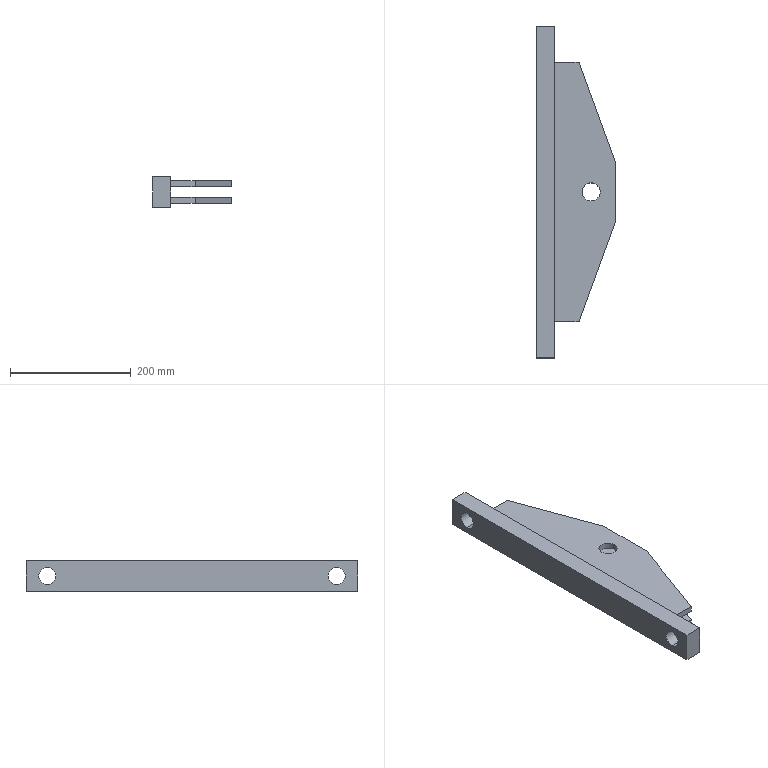Part | SolidWorks | features MBimport 1 | 1 solid | 28 faces | box 130 x 550 x 50 mm | volume 1435918 mm3 | plane 20 | cylinder 8 | commonest cylinder face diameters 28 x4 30 x4
STEP:
#1=CARTESIAN_POINT('',(134.144,275.,-9.181));
#2=VERTEX_POINT('',#1);
#3=CARTESIAN_POINT('',(134.144,275.,-19.181));
#4=VERTEX_POINT('',#3);
#5=CARTESIAN_POINT('',(134.144,275.,24.319));
#6=DIRECTION('',(0.,0.,-1.));
#7=VECTOR('',#6,1000.);
#8=LINE('',#5,#7);
#9=EDGE_CURVE('',#2,#4,#8,.T.);
#10=ORIENTED_EDGE('',*,*,#9,.F.);
#11=CARTESIAN_POINT('',(104.144,275.,-9.181));
#12=VERTEX_POINT('',#11);
#13=CARTESIAN_POINT('',(119.144,275.,-9.181));
#14=DIRECTION('',(0.,0.,1.));
#15=DIRECTION('',(-1.,0.,0.));
#16=AXIS2_PLACEMENT_3D('',#13,#14,#15);
#17=CIRCLE('',#16,15.);
#18=EDGE_CURVE('',#2,#12,#17,.T.);
#19=ORIENTED_EDGE('',*,*,#18,.T.);
#20=CARTESIAN_POINT('',(104.144,275.,-19.181));
#21=VERTEX_POINT('',#20);
#22=CARTESIAN_POINT('',(104.144,275.,24.319));
#23=DIRECTION('',(0.,0.,-1.));
#24=VECTOR('',#23,1000.);
#25=LINE('',#22,#24);
#26=EDGE_CURVE('',#12,#21,#25,.T.);
#27=ORIENTED_EDGE('',*,*,#26,.T.);
#28=CARTESIAN_POINT('',(119.144,275.,-19.181));
#29=DIRECTION('',(0.,0.,1.));
#30=DIRECTION('',(1.,0.,0.));
#31=AXIS2_PLACEMENT_3D('',#28,#29,#30);
#32=CIRCLE('',#31,15.);
#33=EDGE_CURVE('',#4,#21,#32,.T.);
#34=ORIENTED_EDGE('',*,*,#33,.F.);
#35=EDGE_LOOP('',(#10,#19,#27,#34));
#36=FACE_OUTER_BOUND('',#35,.T.);
#37=CARTESIAN_POINT('',(119.144,275.,24.319));
#38=DIRECTION('',(0.,0.,-1.));
#39=DIRECTION('',(-1.,0.,0.));
#40=AXIS2_PLACEMENT_3D('',#37,#38,#39);
#41=CYLINDRICAL_SURFACE('',#40,15.);
#42=ADVANCED_FACE('',(#36),#41,.F.);
#43=CARTESIAN_POINT('',(119.144,275.,-9.181));
#44=DIRECTION('',(0.,0.,1.));
#45=DIRECTION('',(-1.,0.,0.));
#46=AXIS2_PLACEMENT_3D('',#43,#44,#45);
#47=CIRCLE('',#46,15.);
#48=EDGE_CURVE('',#12,#2,#47,.T.);
#49=ORIENTED_EDGE('',*,*,#48,.F.);
#50=ORIENTED_EDGE('',*,*,#18,.F.);
#51=EDGE_LOOP('',(#49,#50));
#52=FACE_BOUND('',#51,.T.);
#53=CARTESIAN_POINT('',(59.144,490.,-9.181));
#54=VERTEX_POINT('',#53);
#55=CARTESIAN_POINT('',(59.144,60.,-9.181));
#56=VERTEX_POINT('',#55);
#57=CARTESIAN_POINT('',(59.144,490.,-9.181));
#58=DIRECTION('',(0.,-1.,0.));
#59=VECTOR('',#58,1000.);
#60=LINE('',#57,#59);
#61=EDGE_CURVE('',#54,#56,#60,.T.);
#62=ORIENTED_EDGE('',*,*,#61,.T.);
#63=CARTESIAN_POINT('',(99.144,60.,-9.181));
#64=VERTEX_POINT('',#63);
#65=CARTESIAN_POINT('',(59.144,60.,-9.181));
#66=DIRECTION('',(1.,0.,0.));
#67=VECTOR('',#66,1000.);
#68=LINE('',#65,#67);
#69=EDGE_CURVE('',#56,#64,#68,.T.);
#70=ORIENTED_EDGE('',*,*,#69,.T.);
#71=CARTESIAN_POINT('',(159.144,225.,-9.181));
#72=VERTEX_POINT('',#71);
#73=CARTESIAN_POINT('',(99.144,60.,-9.181));
#74=DIRECTION('',(0.3417,0.9398,0.));
#75=VECTOR('',#74,1000.);
#76=LINE('',#73,#75);
#77=EDGE_CURVE('',#64,#72,#76,.T.);
#78=ORIENTED_EDGE('',*,*,#77,.T.);
#79=CARTESIAN_POINT('',(159.144,325.,-9.181));
#80=VERTEX_POINT('',#79);
#81=CARTESIAN_POINT('',(159.144,325.,-9.181));
#82=DIRECTION('',(0.,1.,0.));
#83=VECTOR('',#82,1000.);
#84=LINE('',#81,#83);
#85=EDGE_CURVE('',#72,#80,#84,.T.);
#86=ORIENTED_EDGE('',*,*,#85,.T.);
#87=CARTESIAN_POINT('',(99.144,490.,-9.181));
#88=VERTEX_POINT('',#87);
#89=CARTESIAN_POINT('',(99.144,490.,-9.181));
#90=DIRECTION('',(-0.3417,0.9398,0.));
#91=VECTOR('',#90,1000.);
#92=LINE('',#89,#91);
#93=EDGE_CURVE('',#80,#88,#92,.T.);
#94=ORIENTED_EDGE('',*,*,#93,.T.);
#95=CARTESIAN_POINT('',(59.144,490.,-9.181));
#96=DIRECTION('',(-1.,0.,0.));
#97=VECTOR('',#96,1000.);
#98=LINE('',#95,#97);
#99=EDGE_CURVE('',#88,#54,#98,.T.);
#100=ORIENTED_EDGE('',*,*,#99,.T.);
#101=EDGE_LOOP('',(#62,#70,#78,#86,#94,#100));
#102=FACE_OUTER_BOUND('',#101,.T.);
#103=CARTESIAN_POINT('',(0.,0.,-9.181));
#104=DIRECTION('',(0.,0.,-1.));
#105=DIRECTION('',(0.,-1.,0.));
#106=AXIS2_PLACEMENT_3D('',#103,#104,#105);
#107=PLANE('',#106);
#108=ADVANCED_FACE('',(#52,#102),#107,.F.);
#109=CARTESIAN_POINT('',(119.144,275.,-19.181));
#110=DIRECTION('',(0.,0.,1.));
#111=DIRECTION('',(1.,0.,0.));
#112=AXIS2_PLACEMENT_3D('',#109,#110,#111);
#113=CIRCLE('',#112,15.);
#114=EDGE_CURVE('',#21,#4,#113,.T.);
#115=ORIENTED_EDGE('',*,*,#114,.T.);
#116=ORIENTED_EDGE('',*,*,#33,.T.);
#117=EDGE_LOOP('',(#115,#116));
#118=FACE_BOUND('',#117,.T.);
#119=CARTESIAN_POINT('',(59.144,490.,-19.181));
#120=VERTEX_POINT('',#119);
#121=CARTESIAN_POINT('',(59.144,60.,-19.181));
#122=VERTEX_POINT('',#121);
#123=CARTESIAN_POINT('',(59.144,490.,-19.181));
#124=DIRECTION('',(0.,-1.,0.));
#125=VECTOR('',#124,1000.);
#126=LINE('',#123,#125);
#127=EDGE_CURVE('',#120,#122,#126,.T.);
#128=ORIENTED_EDGE('',*,*,#127,.F.);
#129=CARTESIAN_POINT('',(99.144,490.,-19.181));
#130=VERTEX_POINT('',#129);
#131=CARTESIAN_POINT('',(59.144,490.,-19.181));
#132=DIRECTION('',(-1.,0.,0.));
#133=VECTOR('',#132,1000.);
#134=LINE('',#131,#133);
#135=EDGE_CURVE('',#130,#120,#134,.T.);
#136=ORIENTED_EDGE('',*,*,#135,.F.);
#137=CARTESIAN_POINT('',(159.144,325.,-19.181));
#138=VERTEX_POINT('',#137);
#139=CARTESIAN_POINT('',(99.144,490.,-19.181));
#140=DIRECTION('',(-0.3417,0.9398,0.));
#141=VECTOR('',#140,1000.);
#142=LINE('',#139,#141);
#143=EDGE_CURVE('',#138,#130,#142,.T.);
#144=ORIENTED_EDGE('',*,*,#143,.F.);
#145=CARTESIAN_POINT('',(159.144,225.,-19.181));
#146=VERTEX_POINT('',#145);
#147=CARTESIAN_POINT('',(159.144,325.,-19.181));
#148=DIRECTION('',(0.,1.,0.));
#149=VECTOR('',#148,1000.);
#150=LINE('',#147,#149);
#151=EDGE_CURVE('',#146,#138,#150,.T.);
#152=ORIENTED_EDGE('',*,*,#151,.F.);
#153=CARTESIAN_POINT('',(99.144,60.,-19.181));
#154=VERTEX_POINT('',#153);
#155=CARTESIAN_POINT('',(99.144,60.,-19.181));
#156=DIRECTION('',(0.3417,0.9398,0.));
#157=VECTOR('',#156,1000.);
#158=LINE('',#155,#157);
#159=EDGE_CURVE('',#154,#146,#158,.T.);
#160=ORIENTED_EDGE('',*,*,#159,.F.);
#161=CARTESIAN_POINT('',(59.144,60.,-19.181));
#162=DIRECTION('',(1.,0.,0.));
#163=VECTOR('',#162,1000.);
#164=LINE('',#161,#163);
#165=EDGE_CURVE('',#122,#154,#164,.T.);
#166=ORIENTED_EDGE('',*,*,#165,.F.);
#167=EDGE_LOOP('',(#128,#136,#144,#152,#160,#166));
#168=FACE_OUTER_BOUND('',#167,.T.);
#169=CARTESIAN_POINT('',(0.,0.,-19.181));
#170=DIRECTION('',(0.,0.,-1.));
#171=DIRECTION('',(0.,-1.,0.));
#172=AXIS2_PLACEMENT_3D('',#169,#170,#171);
#173=PLANE('',#172);
#174=ADVANCED_FACE('',(#118,#168),#173,.T.);
#175=ORIENTED_EDGE('',*,*,#69,.F.);
#176=CARTESIAN_POINT('',(59.144,60.,-19.181));
#177=DIRECTION('',(0.,0.,1.));
#178=VECTOR('',#177,1000.);
#179=LINE('',#176,#178);
#180=EDGE_CURVE('',#122,#56,#179,.T.);
#181=ORIENTED_EDGE('',*,*,#180,.F.);
#182=ORIENTED_EDGE('',*,*,#165,.T.);
#183=CARTESIAN_POINT('',(99.144,60.,-19.181));
#184=DIRECTION('',(0.,0.,1.));
#185=VECTOR('',#184,1000.);
#186=LINE('',#183,#185);
#187=EDGE_CURVE('',#154,#64,#186,.T.);
#188=ORIENTED_EDGE('',*,*,#187,.T.);
#189=EDGE_LOOP('',(#175,#181,#182,#188));
#190=FACE_OUTER_BOUND('',#189,.T.);
#191=CARTESIAN_POINT('',(59.144,60.,-19.181));
#192=DIRECTION('',(0.,-1.,0.));
#193=DIRECTION('',(0.,0.,-1.));
#194=AXIS2_PLACEMENT_3D('',#191,#192,#193);
#195=PLANE('',#194);
#196=ADVANCED_FACE('',(#190),#195,.T.);
#197=ORIENTED_EDGE('',*,*,#77,.F.);
#198=ORIENTED_EDGE('',*,*,#187,.F.);
#199=ORIENTED_EDGE('',*,*,#159,.T.);
#200=CARTESIAN_POINT('',(159.144,225.,-19.181));
#201=DIRECTION('',(0.,0.,1.));
#202=VECTOR('',#201,1000.);
#203=LINE('',#200,#202);
#204=EDGE_CURVE('',#146,#72,#203,.T.);
#205=ORIENTED_EDGE('',*,*,#204,.T.);
#206=EDGE_LOOP('',(#197,#198,#199,#205));
#207=FACE_OUTER_BOUND('',#206,.T.);
#208=CARTESIAN_POINT('',(99.144,60.,-19.181));
#209=DIRECTION('',(0.9398,-0.3417,0.));
#210=DIRECTION('',(0.,0.,-1.));
#211=AXIS2_PLACEMENT_3D('',#208,#209,#210);
#212=PLANE('',#211);
#213=ADVANCED_FACE('',(#207),#212,.T.);
#214=ORIENTED_EDGE('',*,*,#85,.F.);
#215=ORIENTED_EDGE('',*,*,#204,.F.);
#216=ORIENTED_EDGE('',*,*,#151,.T.);
#217=CARTESIAN_POINT('',(159.144,325.,-19.181));
#218=DIRECTION('',(0.,0.,1.));
#219=VECTOR('',#218,1000.);
#220=LINE('',#217,#219);
#221=EDGE_CURVE('',#138,#80,#220,.T.);
#222=ORIENTED_EDGE('',*,*,#221,.T.);
#223=EDGE_LOOP('',(#214,#215,#216,#222));
#224=FACE_OUTER_BOUND('',#223,.T.);
#225=CARTESIAN_POINT('',(159.144,325.,-19.181));
#226=DIRECTION('',(1.,0.,0.));
#227=DIRECTION('',(0.,1.,0.));
#228=AXIS2_PLACEMENT_3D('',#225,#226,#227);
#229=PLANE('',#228);
#230=ADVANCED_FACE('',(#224),#229,.T.);
#231=ORIENTED_EDGE('',*,*,#93,.F.);
#232=ORIENTED_EDGE('',*,*,#221,.F.);
#233=ORIENTED_EDGE('',*,*,#143,.T.);
#234=CARTESIAN_POINT('',(99.144,490.,-19.181));
#235=DIRECTION('',(0.,0.,1.));
#236=VECTOR('',#235,1000.);
#237=LINE('',#234,#236);
#238=EDGE_CURVE('',#130,#88,#237,.T.);
#239=ORIENTED_EDGE('',*,*,#238,.T.);
#240=EDGE_LOOP('',(#231,#232,#233,#239));
#241=FACE_OUTER_BOUND('',#240,.T.);
#242=CARTESIAN_POINT('',(99.144,490.,-19.181));
#243=DIRECTION('',(0.9398,0.3417,0.));
#244=DIRECTION('',(0.,0.,-1.));
#245=AXIS2_PLACEMENT_3D('',#242,#243,#244);
#246=PLANE('',#245);
#247=ADVANCED_FACE('',(#241),#246,.T.);
#248=ORIENTED_EDGE('',*,*,#99,.F.);
#249=ORIENTED_EDGE('',*,*,#238,.F.);
#250=ORIENTED_EDGE('',*,*,#135,.T.);
#251=CARTESIAN_POINT('',(59.144,490.,-19.181));
#252=DIRECTION('',(0.,0.,1.));
#253=VECTOR('',#252,1000.);
#254=LINE('',#251,#253);
#255=EDGE_CURVE('',#120,#54,#254,.T.);
#256=ORIENTED_EDGE('',*,*,#255,.T.);
#257=EDGE_LOOP('',(#248,#249,#250,#256));
#258=FACE_OUTER_BOUND('',#257,.T.);
#259=CARTESIAN_POINT('',(59.144,490.,-19.181));
#260=DIRECTION('',(0.,1.,0.));
#261=DIRECTION('',(1.,0.,0.));
#262=AXIS2_PLACEMENT_3D('',#259,#260,#261);
#263=PLANE('',#262);
#264=ADVANCED_FACE('',(#258),#263,.T.);
#265=CARTESIAN_POINT('',(104.144,275.,7.819));
#266=VERTEX_POINT('',#265);
#267=CARTESIAN_POINT('',(104.144,275.,17.819));
#268=VERTEX_POINT('',#267);
#269=CARTESIAN_POINT('',(104.144,275.,-25.681));
#270=DIRECTION('',(0.,0.,1.));
#271=VECTOR('',#270,1000.);
#272=LINE('',#269,#271);
#273=EDGE_CURVE('',#266,#268,#272,.T.);
#274=ORIENTED_EDGE('',*,*,#273,.F.);
#275=CARTESIAN_POINT('',(134.144,275.,7.819));
#276=VERTEX_POINT('',#275);
#277=CARTESIAN_POINT('',(119.144,275.,7.819));
#278=DIRECTION('',(0.,0.,1.));
#279=DIRECTION('',(1.,0.,0.));
#280=AXIS2_PLACEMENT_3D('',#277,#278,#279);
#281=CIRCLE('',#280,15.);
#282=EDGE_CURVE('',#276,#266,#281,.T.);
#283=ORIENTED_EDGE('',*,*,#282,.F.);
#284=CARTESIAN_POINT('',(134.144,275.,17.819));
#285=VERTEX_POINT('',#284);
#286=CARTESIAN_POINT('',(134.144,275.,-25.681));
#287=DIRECTION('',(0.,0.,1.));
#288=VECTOR('',#287,1000.);
#289=LINE('',#286,#288);
#290=EDGE_CURVE('',#276,#285,#289,.T.);
#291=ORIENTED_EDGE('',*,*,#290,.T.);
#292=CARTESIAN_POINT('',(119.144,275.,17.819));
#293=DIRECTION('',(0.,0.,1.));
#294=DIRECTION('',(1.,0.,0.));
#295=AXIS2_PLACEMENT_3D('',#292,#293,#294);
#296=CIRCLE('',#295,15.);
#297=EDGE_CURVE('',#285,#268,#296,.T.);
#298=ORIENTED_EDGE('',*,*,#297,.T.);
#299=EDGE_LOOP('',(#274,#283,#291,#298));
#300=FACE_OUTER_BOUND('',#299,.T.);
#301=CARTESIAN_POINT('',(119.144,275.,-25.681));
#302=DIRECTION('',(0.,0.,1.));
#303=DIRECTION('',(1.,0.,0.));
#304=AXIS2_PLACEMENT_3D('',#301,#302,#303);
#305=CYLINDRICAL_SURFACE('',#304,15.);
#306=ADVANCED_FACE('',(#300),#305,.F.);
#307=ORIENTED_EDGE('',*,*,#282,.T.);
#308=CARTESIAN_POINT('',(119.144,275.,7.819));
#309=DIRECTION('',(0.,0.,1.));
#310=DIRECTION('',(1.,0.,0.));
#311=AXIS2_PLACEMENT_3D('',#308,#309,#310);
#312=CIRCLE('',#311,15.);
#313=EDGE_CURVE('',#266,#276,#312,.T.);
#314=ORIENTED_EDGE('',*,*,#313,.T.);
#315=EDGE_LOOP('',(#307,#314));
#316=FACE_BOUND('',#315,.T.);
#317=CARTESIAN_POINT('',(59.144,490.,7.819));
#318=VERTEX_POINT('',#317);
#319=CARTESIAN_POINT('',(59.144,60.,7.819));
#320=VERTEX_POINT('',#319);
#321=CARTESIAN_POINT('',(59.144,490.,7.819));
#322=DIRECTION('',(0.,-1.,0.));
#323=VECTOR('',#322,1000.);
#324=LINE('',#321,#323);
#325=EDGE_CURVE('',#318,#320,#324,.T.);
#326=ORIENTED_EDGE('',*,*,#325,.F.);
#327=CARTESIAN_POINT('',(99.144,490.,7.819));
#328=VERTEX_POINT('',#327);
#329=CARTESIAN_POINT('',(59.144,490.,7.819));
#330=DIRECTION('',(-1.,0.,0.));
#331=VECTOR('',#330,1000.);
#332=LINE('',#329,#331);
#333=EDGE_CURVE('',#328,#318,#332,.T.);
#334=ORIENTED_EDGE('',*,*,#333,.F.);
#335=CARTESIAN_POINT('',(159.144,325.,7.819));
#336=VERTEX_POINT('',#335);
#337=CARTESIAN_POINT('',(99.144,490.,7.819));
#338=DIRECTION('',(-0.3417,0.9398,0.));
#339=VECTOR('',#338,1000.);
#340=LINE('',#337,#339);
#341=EDGE_CURVE('',#336,#328,#340,.T.);
#342=ORIENTED_EDGE('',*,*,#341,.F.);
#343=CARTESIAN_POINT('',(159.144,225.,7.819));
#344=VERTEX_POINT('',#343);
#345=CARTESIAN_POINT('',(159.144,325.,7.819));
#346=DIRECTION('',(0.,1.,0.));
#347=VECTOR('',#346,1000.);
#348=LINE('',#345,#347);
#349=EDGE_CURVE('',#344,#336,#348,.T.);
#350=ORIENTED_EDGE('',*,*,#349,.F.);
#351=CARTESIAN_POINT('',(99.144,60.,7.819));
#352=VERTEX_POINT('',#351);
#353=CARTESIAN_POINT('',(99.144,60.,7.819));
#354=DIRECTION('',(0.3417,0.9398,0.));
#355=VECTOR('',#354,1000.);
#356=LINE('',#353,#355);
#357=EDGE_CURVE('',#352,#344,#356,.T.);
#358=ORIENTED_EDGE('',*,*,#357,.F.);
#359=CARTESIAN_POINT('',(59.144,60.,7.819));
#360=DIRECTION('',(1.,0.,0.));
#361=VECTOR('',#360,1000.);
#362=LINE('',#359,#361);
#363=EDGE_CURVE('',#320,#352,#362,.T.);
#364=ORIENTED_EDGE('',*,*,#363,.F.);
#365=EDGE_LOOP('',(#326,#334,#342,#350,#358,#364));
#366=FACE_OUTER_BOUND('',#365,.T.);
#367=CARTESIAN_POINT('',(0.,0.,7.819));
#368=DIRECTION('',(0.,0.,1.));
#369=DIRECTION('',(1.,0.,0.));
#370=AXIS2_PLACEMENT_3D('',#367,#368,#369);
#371=PLANE('',#370);
#372=ADVANCED_FACE('',(#316,#366),#371,.F.);
#373=ORIENTED_EDGE('',*,*,#297,.F.);
#374=CARTESIAN_POINT('',(119.144,275.,17.819));
#375=DIRECTION('',(0.,0.,1.));
#376=DIRECTION('',(1.,0.,0.));
#377=AXIS2_PLACEMENT_3D('',#374,#375,#376);
#378=CIRCLE('',#377,15.);
#379=EDGE_CURVE('',#268,#285,#378,.T.);
#380=ORIENTED_EDGE('',*,*,#379,.F.);
#381=EDGE_LOOP('',(#373,#380));
#382=FACE_BOUND('',#381,.T.);
#383=CARTESIAN_POINT('',(59.144,490.,17.819));
#384=VERTEX_POINT('',#383);
#385=CARTESIAN_POINT('',(59.144,60.,17.819));
#386=VERTEX_POINT('',#385);
#387=CARTESIAN_POINT('',(59.144,490.,17.819));
#388=DIRECTION('',(0.,-1.,0.));
#389=VECTOR('',#388,1000.);
#390=LINE('',#387,#389);
#391=EDGE_CURVE('',#384,#386,#390,.T.);
#392=ORIENTED_EDGE('',*,*,#391,.T.);
#393=CARTESIAN_POINT('',(99.144,60.,17.819));
#394=VERTEX_POINT('',#393);
#395=CARTESIAN_POINT('',(59.144,60.,17.819));
#396=DIRECTION('',(1.,0.,0.));
#397=VECTOR('',#396,1000.);
#398=LINE('',#395,#397);
#399=EDGE_CURVE('',#386,#394,#398,.T.);
#400=ORIENTED_EDGE('',*,*,#399,.T.);
#401=CARTESIAN_POINT('',(159.144,225.,17.819));
#402=VERTEX_POINT('',#401);
#403=CARTESIAN_POINT('',(99.144,60.,17.819));
#404=DIRECTION('',(0.3417,0.9398,0.));
#405=VECTOR('',#404,1000.);
#406=LINE('',#403,#405);
#407=EDGE_CURVE('',#394,#402,#406,.T.);
#408=ORIENTED_EDGE('',*,*,#407,.T.);
#409=CARTESIAN_POINT('',(159.144,325.,17.819));
#410=VERTEX_POINT('',#409);
#411=CARTESIAN_POINT('',(159.144,325.,17.819));
#412=DIRECTION('',(0.,1.,0.));
#413=VECTOR('',#412,1000.);
#414=LINE('',#411,#413);
#415=EDGE_CURVE('',#402,#410,#414,.T.);
#416=ORIENTED_EDGE('',*,*,#415,.T.);
#417=CARTESIAN_POINT('',(99.144,490.,17.819));
#418=VERTEX_POINT('',#417);
#419=CARTESIAN_POINT('',(99.144,490.,17.819));
#420=DIRECTION('',(-0.3417,0.9398,0.));
#421=VECTOR('',#420,1000.);
#422=LINE('',#419,#421);
#423=EDGE_CURVE('',#410,#418,#422,.T.);
#424=ORIENTED_EDGE('',*,*,#423,.T.);
#425=CARTESIAN_POINT('',(59.144,490.,17.819));
#426=DIRECTION('',(-1.,0.,0.));
#427=VECTOR('',#426,1000.);
#428=LINE('',#425,#427);
#429=EDGE_CURVE('',#418,#384,#428,.T.);
#430=ORIENTED_EDGE('',*,*,#429,.T.);
#431=EDGE_LOOP('',(#392,#400,#408,#416,#424,#430));
#432=FACE_OUTER_BOUND('',#431,.T.);
#433=CARTESIAN_POINT('',(0.,0.,17.819));
#434=DIRECTION('',(0.,0.,1.));
#435=DIRECTION('',(1.,0.,0.));
#436=AXIS2_PLACEMENT_3D('',#433,#434,#435);
#437=PLANE('',#436);
#438=ADVANCED_FACE('',(#382,#432),#437,.T.);
#439=ORIENTED_EDGE('',*,*,#333,.T.);
#440=CARTESIAN_POINT('',(59.144,490.,17.819));
#441=DIRECTION('',(0.,0.,-1.));
#442=VECTOR('',#441,1000.);
#443=LINE('',#440,#442);
#444=EDGE_CURVE('',#384,#318,#443,.T.);
#445=ORIENTED_EDGE('',*,*,#444,.F.);
#446=ORIENTED_EDGE('',*,*,#429,.F.);
#447=CARTESIAN_POINT('',(99.144,490.,17.819));
#448=DIRECTION('',(0.,0.,-1.));
#449=VECTOR('',#448,1000.);
#450=LINE('',#447,#449);
#451=EDGE_CURVE('',#418,#328,#450,.T.);
#452=ORIENTED_EDGE('',*,*,#451,.T.);
#453=EDGE_LOOP('',(#439,#445,#446,#452));
#454=FACE_OUTER_BOUND('',#453,.T.);
#455=CARTESIAN_POINT('',(59.144,490.,17.819));
#456=DIRECTION('',(0.,-1.,0.));
#457=DIRECTION('',(0.,0.,-1.));
#458=AXIS2_PLACEMENT_3D('',#455,#456,#457);
#459=PLANE('',#458);
#460=ADVANCED_FACE('',(#454),#459,.F.);
#461=ORIENTED_EDGE('',*,*,#341,.T.);
#462=ORIENTED_EDGE('',*,*,#451,.F.);
#463=ORIENTED_EDGE('',*,*,#423,.F.);
#464=CARTESIAN_POINT('',(159.144,325.,17.819));
#465=DIRECTION('',(0.,0.,-1.));
#466=VECTOR('',#465,1000.);
#467=LINE('',#464,#466);
#468=EDGE_CURVE('',#410,#336,#467,.T.);
#469=ORIENTED_EDGE('',*,*,#468,.T.);
#470=EDGE_LOOP('',(#461,#462,#463,#469));
#471=FACE_OUTER_BOUND('',#470,.T.);
#472=CARTESIAN_POINT('',(99.144,490.,17.819));
#473=DIRECTION('',(-0.9398,-0.3417,0.));
#474=DIRECTION('',(-0.3417,0.9398,0.));
#475=AXIS2_PLACEMENT_3D('',#472,#473,#474);
#476=PLANE('',#475);
#477=ADVANCED_FACE('',(#471),#476,.F.);
#478=ORIENTED_EDGE('',*,*,#349,.T.);
#479=ORIENTED_EDGE('',*,*,#468,.F.);
#480=ORIENTED_EDGE('',*,*,#415,.F.);
#481=CARTESIAN_POINT('',(159.144,225.,17.819));
#482=DIRECTION('',(0.,0.,-1.));
#483=VECTOR('',#482,1000.);
#484=LINE('',#481,#483);
#485=EDGE_CURVE('',#402,#344,#484,.T.);
#486=ORIENTED_EDGE('',*,*,#485,.T.);
#487=EDGE_LOOP('',(#478,#479,#480,#486));
#488=FACE_OUTER_BOUND('',#487,.T.);
#489=CARTESIAN_POINT('',(159.144,325.,17.819));
#490=DIRECTION('',(-1.,0.,0.));
#491=DIRECTION('',(0.,0.,1.));
#492=AXIS2_PLACEMENT_3D('',#489,#490,#491);
#493=PLANE('',#492);
#494=ADVANCED_FACE('',(#488),#493,.F.);
#495=ORIENTED_EDGE('',*,*,#357,.T.);
#496=ORIENTED_EDGE('',*,*,#485,.F.);
#497=ORIENTED_EDGE('',*,*,#407,.F.);
#498=CARTESIAN_POINT('',(99.144,60.,17.819));
#499=DIRECTION('',(0.,0.,-1.));
#500=VECTOR('',#499,1000.);
#501=LINE('',#498,#500);
#502=EDGE_CURVE('',#394,#352,#501,.T.);
#503=ORIENTED_EDGE('',*,*,#502,.T.);
#504=EDGE_LOOP('',(#495,#496,#497,#503));
#505=FACE_OUTER_BOUND('',#504,.T.);
#506=CARTESIAN_POINT('',(99.144,60.,17.819));
#507=DIRECTION('',(-0.9398,0.3417,0.));
#508=DIRECTION('',(0.,0.,1.));
#509=AXIS2_PLACEMENT_3D('',#506,#507,#508);
#510=PLANE('',#509);
#511=ADVANCED_FACE('',(#505),#510,.F.);
#512=ORIENTED_EDGE('',*,*,#363,.T.);
#513=ORIENTED_EDGE('',*,*,#502,.F.);
#514=ORIENTED_EDGE('',*,*,#399,.F.);
#515=CARTESIAN_POINT('',(59.144,60.,17.819));
#516=DIRECTION('',(0.,0.,-1.));
#517=VECTOR('',#516,1000.);
#518=LINE('',#515,#517);
#519=EDGE_CURVE('',#386,#320,#518,.T.);
#520=ORIENTED_EDGE('',*,*,#519,.T.);
#521=EDGE_LOOP('',(#512,#513,#514,#520));
#522=FACE_OUTER_BOUND('',#521,.T.);
#523=CARTESIAN_POINT('',(59.144,60.,17.819));
#524=DIRECTION('',(0.,1.,0.));
#525=DIRECTION('',(1.,0.,0.));
#526=AXIS2_PLACEMENT_3D('',#523,#524,#525);
#527=PLANE('',#526);
#528=ADVANCED_FACE('',(#522),#527,.F.);
#529=CARTESIAN_POINT('',(29.144,515.,13.319));
#530=VERTEX_POINT('',#529);
#531=CARTESIAN_POINT('',(59.144,515.,13.319));
#532=VERTEX_POINT('',#531);
#533=CARTESIAN_POINT('',(29.144,515.,13.319));
#534=DIRECTION('',(1.,0.,0.));
#535=VECTOR('',#534,1000.);
#536=LINE('',#533,#535);
#537=EDGE_CURVE('',#530,#532,#536,.T.);
#538=ORIENTED_EDGE('',*,*,#537,.F.);
#539=CARTESIAN_POINT('',(29.144,515.,-14.681));
#540=VERTEX_POINT('',#539);
#541=CARTESIAN_POINT('',(29.144,515.,-0.6806));
#542=DIRECTION('',(1.,0.,0.));
#543=DIRECTION('',(0.,0.,-1.));
#544=AXIS2_PLACEMENT_3D('',#541,#542,#543);
#545=CIRCLE('',#544,14.);
#546=EDGE_CURVE('',#540,#530,#545,.T.);
#547=ORIENTED_EDGE('',*,*,#546,.F.);
#548=CARTESIAN_POINT('',(59.144,515.,-14.681));
#549=VERTEX_POINT('',#548);
#550=CARTESIAN_POINT('',(29.144,515.,-14.681));
#551=DIRECTION('',(1.,0.,0.));
#552=VECTOR('',#551,1000.);
#553=LINE('',#550,#552);
#554=EDGE_CURVE('',#540,#549,#553,.T.);
#555=ORIENTED_EDGE('',*,*,#554,.T.);
#556=CARTESIAN_POINT('',(59.144,515.,-0.6806));
#557=DIRECTION('',(1.,0.,0.));
#558=DIRECTION('',(0.,0.,-1.));
#559=AXIS2_PLACEMENT_3D('',#556,#557,#558);
#560=CIRCLE('',#559,14.);
#561=EDGE_CURVE('',#549,#532,#560,.T.);
#562=ORIENTED_EDGE('',*,*,#561,.T.);
#563=EDGE_LOOP('',(#538,#547,#555,#562));
#564=FACE_OUTER_BOUND('',#563,.T.);
#565=CARTESIAN_POINT('',(29.144,515.,-0.6806));
#566=DIRECTION('',(1.,0.,0.));
#567=DIRECTION('',(0.,0.,-1.));
#568=AXIS2_PLACEMENT_3D('',#565,#566,#567);
#569=CYLINDRICAL_SURFACE('',#568,14.);
#570=ADVANCED_FACE('',(#564),#569,.F.);
#571=CARTESIAN_POINT('',(29.144,35.,13.319));
#572=VERTEX_POINT('',#571);
#573=CARTESIAN_POINT('',(59.144,35.,13.319));
#574=VERTEX_POINT('',#573);
#575=CARTESIAN_POINT('',(29.144,35.,13.319));
#576=DIRECTION('',(1.,0.,0.));
#577=VECTOR('',#576,1000.);
#578=LINE('',#575,#577);
#579=EDGE_CURVE('',#572,#574,#578,.T.);
#580=ORIENTED_EDGE('',*,*,#579,.F.);
#581=CARTESIAN_POINT('',(29.144,35.,-14.681));
#582=VERTEX_POINT('',#581);
#583=CARTESIAN_POINT('',(29.144,35.,-0.6806));
#584=DIRECTION('',(1.,0.,0.));
#585=DIRECTION('',(0.,0.,-1.));
#586=AXIS2_PLACEMENT_3D('',#583,#584,#585);
#587=CIRCLE('',#586,14.);
#588=EDGE_CURVE('',#582,#572,#587,.T.);
#589=ORIENTED_EDGE('',*,*,#588,.F.);
#590=CARTESIAN_POINT('',(59.144,35.,-14.681));
#591=VERTEX_POINT('',#590);
#592=CARTESIAN_POINT('',(29.144,35.,-14.681));
#593=DIRECTION('',(1.,0.,0.));
#594=VECTOR('',#593,1000.);
#595=LINE('',#592,#594);
#596=EDGE_CURVE('',#582,#591,#595,.T.);
#597=ORIENTED_EDGE('',*,*,#596,.T.);
#598=CARTESIAN_POINT('',(59.144,35.,-0.6806));
#599=DIRECTION('',(1.,0.,0.));
#600=DIRECTION('',(0.,0.,-1.));
#601=AXIS2_PLACEMENT_3D('',#598,#599,#600);
#602=CIRCLE('',#601,14.);
#603=EDGE_CURVE('',#591,#574,#602,.T.);
#604=ORIENTED_EDGE('',*,*,#603,.T.);
#605=EDGE_LOOP('',(#580,#589,#597,#604));
#606=FACE_OUTER_BOUND('',#605,.T.);
#607=CARTESIAN_POINT('',(29.144,35.,-0.6806));
#608=DIRECTION('',(1.,0.,0.));
#609=DIRECTION('',(0.,0.,-1.));
#610=AXIS2_PLACEMENT_3D('',#607,#608,#609);
#611=CYLINDRICAL_SURFACE('',#610,14.);
#612=ADVANCED_FACE('',(#606),#611,.F.);
#613=CARTESIAN_POINT('',(29.144,0.,-25.681));
#614=VERTEX_POINT('',#613);
#615=CARTESIAN_POINT('',(29.144,0.,24.319));
#616=VERTEX_POINT('',#615);
#617=CARTESIAN_POINT('',(29.144,0.,-25.681));
#618=DIRECTION('',(0.,0.,1.));
#619=VECTOR('',#618,1000.);
#620=LINE('',#617,#619);
#621=EDGE_CURVE('',#614,#616,#620,.T.);
#622=ORIENTED_EDGE('',*,*,#621,.F.);
#623=CARTESIAN_POINT('',(59.144,0.,-25.681));
#624=VERTEX_POINT('',#623);
#625=CARTESIAN_POINT('',(29.144,0.,-25.681));
#626=DIRECTION('',(-1.,0.,0.));
#627=VECTOR('',#626,1000.);
#628=LINE('',#625,#627);
#629=EDGE_CURVE('',#624,#614,#628,.T.);
#630=ORIENTED_EDGE('',*,*,#629,.F.);
#631=CARTESIAN_POINT('',(59.144,0.,24.319));
#632=VERTEX_POINT('',#631);
#633=CARTESIAN_POINT('',(59.144,0.,-25.681));
#634=DIRECTION('',(0.,0.,-1.));
#635=VECTOR('',#634,1000.);
#636=LINE('',#633,#635);
#637=EDGE_CURVE('',#632,#624,#636,.T.);
#638=ORIENTED_EDGE('',*,*,#637,.F.);
#639=CARTESIAN_POINT('',(29.144,0.,24.319));
#640=DIRECTION('',(1.,0.,0.));
#641=VECTOR('',#640,1000.);
#642=LINE('',#639,#641);
#643=EDGE_CURVE('',#616,#632,#642,.T.);
#644=ORIENTED_EDGE('',*,*,#643,.F.);
#645=EDGE_LOOP('',(#622,#630,#638,#644));
#646=FACE_OUTER_BOUND('',#645,.T.);
#647=CARTESIAN_POINT('',(0.,0.,0.));
#648=DIRECTION('',(0.,1.,0.));
#649=DIRECTION('',(1.,0.,0.));
#650=AXIS2_PLACEMENT_3D('',#647,#648,#649);
#651=PLANE('',#650);
#652=ADVANCED_FACE('',(#646),#651,.F.);
#653=CARTESIAN_POINT('',(29.144,550.,-25.681));
#654=VERTEX_POINT('',#653);
#655=CARTESIAN_POINT('',(29.144,550.,24.319));
#656=VERTEX_POINT('',#655);
#657=CARTESIAN_POINT('',(29.144,550.,-25.681));
#658=DIRECTION('',(0.,0.,1.));
#659=VECTOR('',#658,1000.);
#660=LINE('',#657,#659);
#661=EDGE_CURVE('',#654,#656,#660,.T.);
#662=ORIENTED_EDGE('',*,*,#661,.T.);
#663=CARTESIAN_POINT('',(59.144,550.,24.319));
#664=VERTEX_POINT('',#663);
#665=CARTESIAN_POINT('',(29.144,550.,24.319));
#666=DIRECTION('',(1.,0.,0.));
#667=VECTOR('',#666,1000.);
#668=LINE('',#665,#667);
#669=EDGE_CURVE('',#656,#664,#668,.T.);
#670=ORIENTED_EDGE('',*,*,#669,.T.);
#671=CARTESIAN_POINT('',(59.144,550.,-25.681));
#672=VERTEX_POINT('',#671);
#673=CARTESIAN_POINT('',(59.144,550.,-25.681));
#674=DIRECTION('',(0.,0.,-1.));
#675=VECTOR('',#674,1000.);
#676=LINE('',#673,#675);
#677=EDGE_CURVE('',#664,#672,#676,.T.);
#678=ORIENTED_EDGE('',*,*,#677,.T.);
#679=CARTESIAN_POINT('',(29.144,550.,-25.681));
#680=DIRECTION('',(-1.,0.,0.));
#681=VECTOR('',#680,1000.);
#682=LINE('',#679,#681);
#683=EDGE_CURVE('',#672,#654,#682,.T.);
#684=ORIENTED_EDGE('',*,*,#683,.T.);
#685=EDGE_LOOP('',(#662,#670,#678,#684));
#686=FACE_OUTER_BOUND('',#685,.T.);
#687=CARTESIAN_POINT('',(0.,550.,0.));
#688=DIRECTION('',(0.,1.,0.));
#689=DIRECTION('',(1.,0.,0.));
#690=AXIS2_PLACEMENT_3D('',#687,#688,#689);
#691=PLANE('',#690);
#692=ADVANCED_FACE('',(#686),#691,.T.);
#693=ORIENTED_EDGE('',*,*,#629,.T.);
#694=CARTESIAN_POINT('',(29.144,550.,-25.681));
#695=DIRECTION('',(0.,-1.,0.));
#696=VECTOR('',#695,1000.);
#697=LINE('',#694,#696);
#698=EDGE_CURVE('',#654,#614,#697,.T.);
#699=ORIENTED_EDGE('',*,*,#698,.F.);
#700=ORIENTED_EDGE('',*,*,#683,.F.);
#701=CARTESIAN_POINT('',(59.144,550.,-25.681));
#702=DIRECTION('',(0.,-1.,0.));
#703=VECTOR('',#702,1000.);
#704=LINE('',#701,#703);
#705=EDGE_CURVE('',#672,#624,#704,.T.);
#706=ORIENTED_EDGE('',*,*,#705,.T.);
#707=EDGE_LOOP('',(#693,#699,#700,#706));
#708=FACE_OUTER_BOUND('',#707,.T.);
#709=CARTESIAN_POINT('',(29.144,550.,-25.681));
#710=DIRECTION('',(0.,0.,1.));
#711=DIRECTION('',(1.,0.,0.));
#712=AXIS2_PLACEMENT_3D('',#709,#710,#711);
#713=PLANE('',#712);
#714=ADVANCED_FACE('',(#708),#713,.F.);
#715=ORIENTED_EDGE('',*,*,#603,.F.);
#716=CARTESIAN_POINT('',(59.144,35.,-0.6806));
#717=DIRECTION('',(1.,0.,0.));
#718=DIRECTION('',(0.,0.,-1.));
#719=AXIS2_PLACEMENT_3D('',#716,#717,#718);
#720=CIRCLE('',#719,14.);
#721=EDGE_CURVE('',#574,#591,#720,.T.);
#722=ORIENTED_EDGE('',*,*,#721,.F.);
#723=EDGE_LOOP('',(#715,#722));
#724=FACE_BOUND('',#723,.T.);
#725=ORIENTED_EDGE('',*,*,#561,.F.);
#726=CARTESIAN_POINT('',(59.144,515.,-0.6806));
#727=DIRECTION('',(1.,0.,0.));
#728=DIRECTION('',(0.,0.,-1.));
#729=AXIS2_PLACEMENT_3D('',#726,#727,#728);
#730=CIRCLE('',#729,14.);
#731=EDGE_CURVE('',#532,#549,#730,.T.);
#732=ORIENTED_EDGE('',*,*,#731,.F.);
#733=EDGE_LOOP('',(#725,#732));
#734=FACE_BOUND('',#733,.T.);
#735=ORIENTED_EDGE('',*,*,#519,.F.);
#736=ORIENTED_EDGE('',*,*,#391,.F.);
#737=ORIENTED_EDGE('',*,*,#444,.T.);
#738=ORIENTED_EDGE('',*,*,#325,.T.);
#739=EDGE_LOOP('',(#735,#736,#737,#738));
#740=FACE_BOUND('',#739,.T.);
#741=ORIENTED_EDGE('',*,*,#255,.F.);
#742=ORIENTED_EDGE('',*,*,#127,.T.);
#743=ORIENTED_EDGE('',*,*,#180,.T.);
#744=ORIENTED_EDGE('',*,*,#61,.F.);
#745=EDGE_LOOP('',(#741,#742,#743,#744));
#746=FACE_BOUND('',#745,.T.);
#747=ORIENTED_EDGE('',*,*,#637,.T.);
#748=ORIENTED_EDGE('',*,*,#705,.F.);
#749=ORIENTED_EDGE('',*,*,#677,.F.);
#750=CARTESIAN_POINT('',(59.144,550.,24.319));
#751=DIRECTION('',(0.,-1.,0.));
#752=VECTOR('',#751,1000.);
#753=LINE('',#750,#752);
#754=EDGE_CURVE('',#664,#632,#753,.T.);
#755=ORIENTED_EDGE('',*,*,#754,.T.);
#756=EDGE_LOOP('',(#747,#748,#749,#755));
#757=FACE_OUTER_BOUND('',#756,.T.);
#758=CARTESIAN_POINT('',(59.144,550.,-25.681));
#759=DIRECTION('',(-1.,0.,0.));
#760=DIRECTION('',(0.,1.,0.));
#761=AXIS2_PLACEMENT_3D('',#758,#759,#760);
#762=PLANE('',#761);
#763=ADVANCED_FACE('',(#724,#734,#740,#746,#757),#762,.F.);
#764=ORIENTED_EDGE('',*,*,#643,.T.);
#765=ORIENTED_EDGE('',*,*,#754,.F.);
#766=ORIENTED_EDGE('',*,*,#669,.F.);
#767=CARTESIAN_POINT('',(29.144,550.,24.319));
#768=DIRECTION('',(0.,-1.,0.));
#769=VECTOR('',#768,1000.);
#770=LINE('',#767,#769);
#771=EDGE_CURVE('',#656,#616,#770,.T.);
#772=ORIENTED_EDGE('',*,*,#771,.T.);
#773=EDGE_LOOP('',(#764,#765,#766,#772));
#774=FACE_OUTER_BOUND('',#773,.T.);
#775=CARTESIAN_POINT('',(29.144,550.,24.319));
#776=DIRECTION('',(0.,0.,-1.));
#777=DIRECTION('',(0.,-1.,0.));
#778=AXIS2_PLACEMENT_3D('',#775,#776,#777);
#779=PLANE('',#778);
#780=ADVANCED_FACE('',(#774),#779,.F.);
#781=ORIENTED_EDGE('',*,*,#588,.T.);
#782=CARTESIAN_POINT('',(29.144,35.,-0.6806));
#783=DIRECTION('',(1.,0.,0.));
#784=DIRECTION('',(0.,0.,-1.));
#785=AXIS2_PLACEMENT_3D('',#782,#783,#784);
#786=CIRCLE('',#785,14.);
#787=EDGE_CURVE('',#572,#582,#786,.T.);
#788=ORIENTED_EDGE('',*,*,#787,.T.);
#789=EDGE_LOOP('',(#781,#788));
#790=FACE_BOUND('',#789,.T.);
#791=ORIENTED_EDGE('',*,*,#546,.T.);
#792=CARTESIAN_POINT('',(29.144,515.,-0.6806));
#793=DIRECTION('',(1.,0.,0.));
#794=DIRECTION('',(0.,0.,-1.));
#795=AXIS2_PLACEMENT_3D('',#792,#793,#794);
#796=CIRCLE('',#795,14.);
#797=EDGE_CURVE('',#530,#540,#796,.T.);
#798=ORIENTED_EDGE('',*,*,#797,.T.);
#799=EDGE_LOOP('',(#791,#798));
#800=FACE_BOUND('',#799,.T.);
#801=ORIENTED_EDGE('',*,*,#621,.T.);
#802=ORIENTED_EDGE('',*,*,#771,.F.);
#803=ORIENTED_EDGE('',*,*,#661,.F.);
#804=ORIENTED_EDGE('',*,*,#698,.T.);
#805=EDGE_LOOP('',(#801,#802,#803,#804));
#806=FACE_OUTER_BOUND('',#805,.T.);
#807=CARTESIAN_POINT('',(29.144,550.,-25.681));
#808=DIRECTION('',(1.,0.,0.));
#809=DIRECTION('',(0.,0.,-1.));
#810=AXIS2_PLACEMENT_3D('',#807,#808,#809);
#811=PLANE('',#810);
#812=ADVANCED_FACE('',(#790,#800,#806),#811,.F.);
#813=ORIENTED_EDGE('',*,*,#787,.F.);
#814=ORIENTED_EDGE('',*,*,#579,.T.);
#815=ORIENTED_EDGE('',*,*,#721,.T.);
#816=ORIENTED_EDGE('',*,*,#596,.F.);
#817=EDGE_LOOP('',(#813,#814,#815,#816));
#818=FACE_OUTER_BOUND('',#817,.T.);
#819=CARTESIAN_POINT('',(29.144,35.,-0.6806));
#820=DIRECTION('',(1.,0.,0.));
#821=DIRECTION('',(0.,0.,-1.));
#822=AXIS2_PLACEMENT_3D('',#819,#820,#821);
#823=CYLINDRICAL_SURFACE('',#822,14.);
#824=ADVANCED_FACE('',(#818),#823,.F.);
#825=ORIENTED_EDGE('',*,*,#797,.F.);
#826=ORIENTED_EDGE('',*,*,#537,.T.);
#827=ORIENTED_EDGE('',*,*,#731,.T.);
#828=ORIENTED_EDGE('',*,*,#554,.F.);
#829=EDGE_LOOP('',(#825,#826,#827,#828));
#830=FACE_OUTER_BOUND('',#829,.T.);
#831=CARTESIAN_POINT('',(29.144,515.,-0.6806));
#832=DIRECTION('',(1.,0.,0.));
#833=DIRECTION('',(0.,0.,-1.));
#834=AXIS2_PLACEMENT_3D('',#831,#832,#833);
#835=CYLINDRICAL_SURFACE('',#834,14.);
#836=ADVANCED_FACE('',(#830),#835,.F.);
#837=ORIENTED_EDGE('',*,*,#313,.F.);
#838=ORIENTED_EDGE('',*,*,#273,.T.);
#839=ORIENTED_EDGE('',*,*,#379,.T.);
#840=ORIENTED_EDGE('',*,*,#290,.F.);
#841=EDGE_LOOP('',(#837,#838,#839,#840));
#842=FACE_OUTER_BOUND('',#841,.T.);
#843=CARTESIAN_POINT('',(119.144,275.,-25.681));
#844=DIRECTION('',(0.,0.,1.));
#845=DIRECTION('',(1.,0.,0.));
#846=AXIS2_PLACEMENT_3D('',#843,#844,#845);
#847=CYLINDRICAL_SURFACE('',#846,15.);
#848=ADVANCED_FACE('',(#842),#847,.F.);
#849=ORIENTED_EDGE('',*,*,#48,.T.);
#850=ORIENTED_EDGE('',*,*,#9,.T.);
#851=ORIENTED_EDGE('',*,*,#114,.F.);
#852=ORIENTED_EDGE('',*,*,#26,.F.);
#853=EDGE_LOOP('',(#849,#850,#851,#852));
#854=FACE_OUTER_BOUND('',#853,.T.);
#855=CARTESIAN_POINT('',(119.144,275.,24.319));
#856=DIRECTION('',(0.,0.,-1.));
#857=DIRECTION('',(-1.,0.,0.));
#858=AXIS2_PLACEMENT_3D('',#855,#856,#857);
#859=CYLINDRICAL_SURFACE('',#858,15.);
#860=ADVANCED_FACE('',(#854),#859,.F.);
#861=CLOSED_SHELL('',(#42,#108,#174,#196,#213,#230,#247,#264,#306,#372,#438,#460,#477,#494,#511,#528,#570,#612,#652,#692,#714,#763,#780,#812,#824,#836,#848,#860));
#862=MANIFOLD_SOLID_BREP('',#861);
#863=CARTESIAN_POINT('',(0.,0.,0.));
#864=DIRECTION('',(0.,0.,1.));
#865=DIRECTION('',(1.,0.,0.));
#866=AXIS2_PLACEMENT_3D('',#863,#864,#865);
#867=(LENGTH_UNIT()NAMED_UNIT(*)SI_UNIT(.MILLI.,.METRE.));
#868=UNCERTAINTY_MEASURE_WITH_UNIT(LENGTH_MEASURE(0.00001),#867,'','');
#869=(NAMED_UNIT(*)PLANE_ANGLE_UNIT()SI_UNIT($,.RADIAN.));
#870=(NAMED_UNIT(*)SI_UNIT($,.STERADIAN.)SOLID_ANGLE_UNIT());
#871=(GEOMETRIC_REPRESENTATION_CONTEXT(3)GLOBAL_UNCERTAINTY_ASSIGNED_CONTEXT((#868))GLOBAL_UNIT_ASSIGNED_CONTEXT((#867,#869,#870))REPRESENTATION_CONTEXT('',''));
#872=ADVANCED_BREP_SHAPE_REPRESENTATION('',(#862,#866),#871);